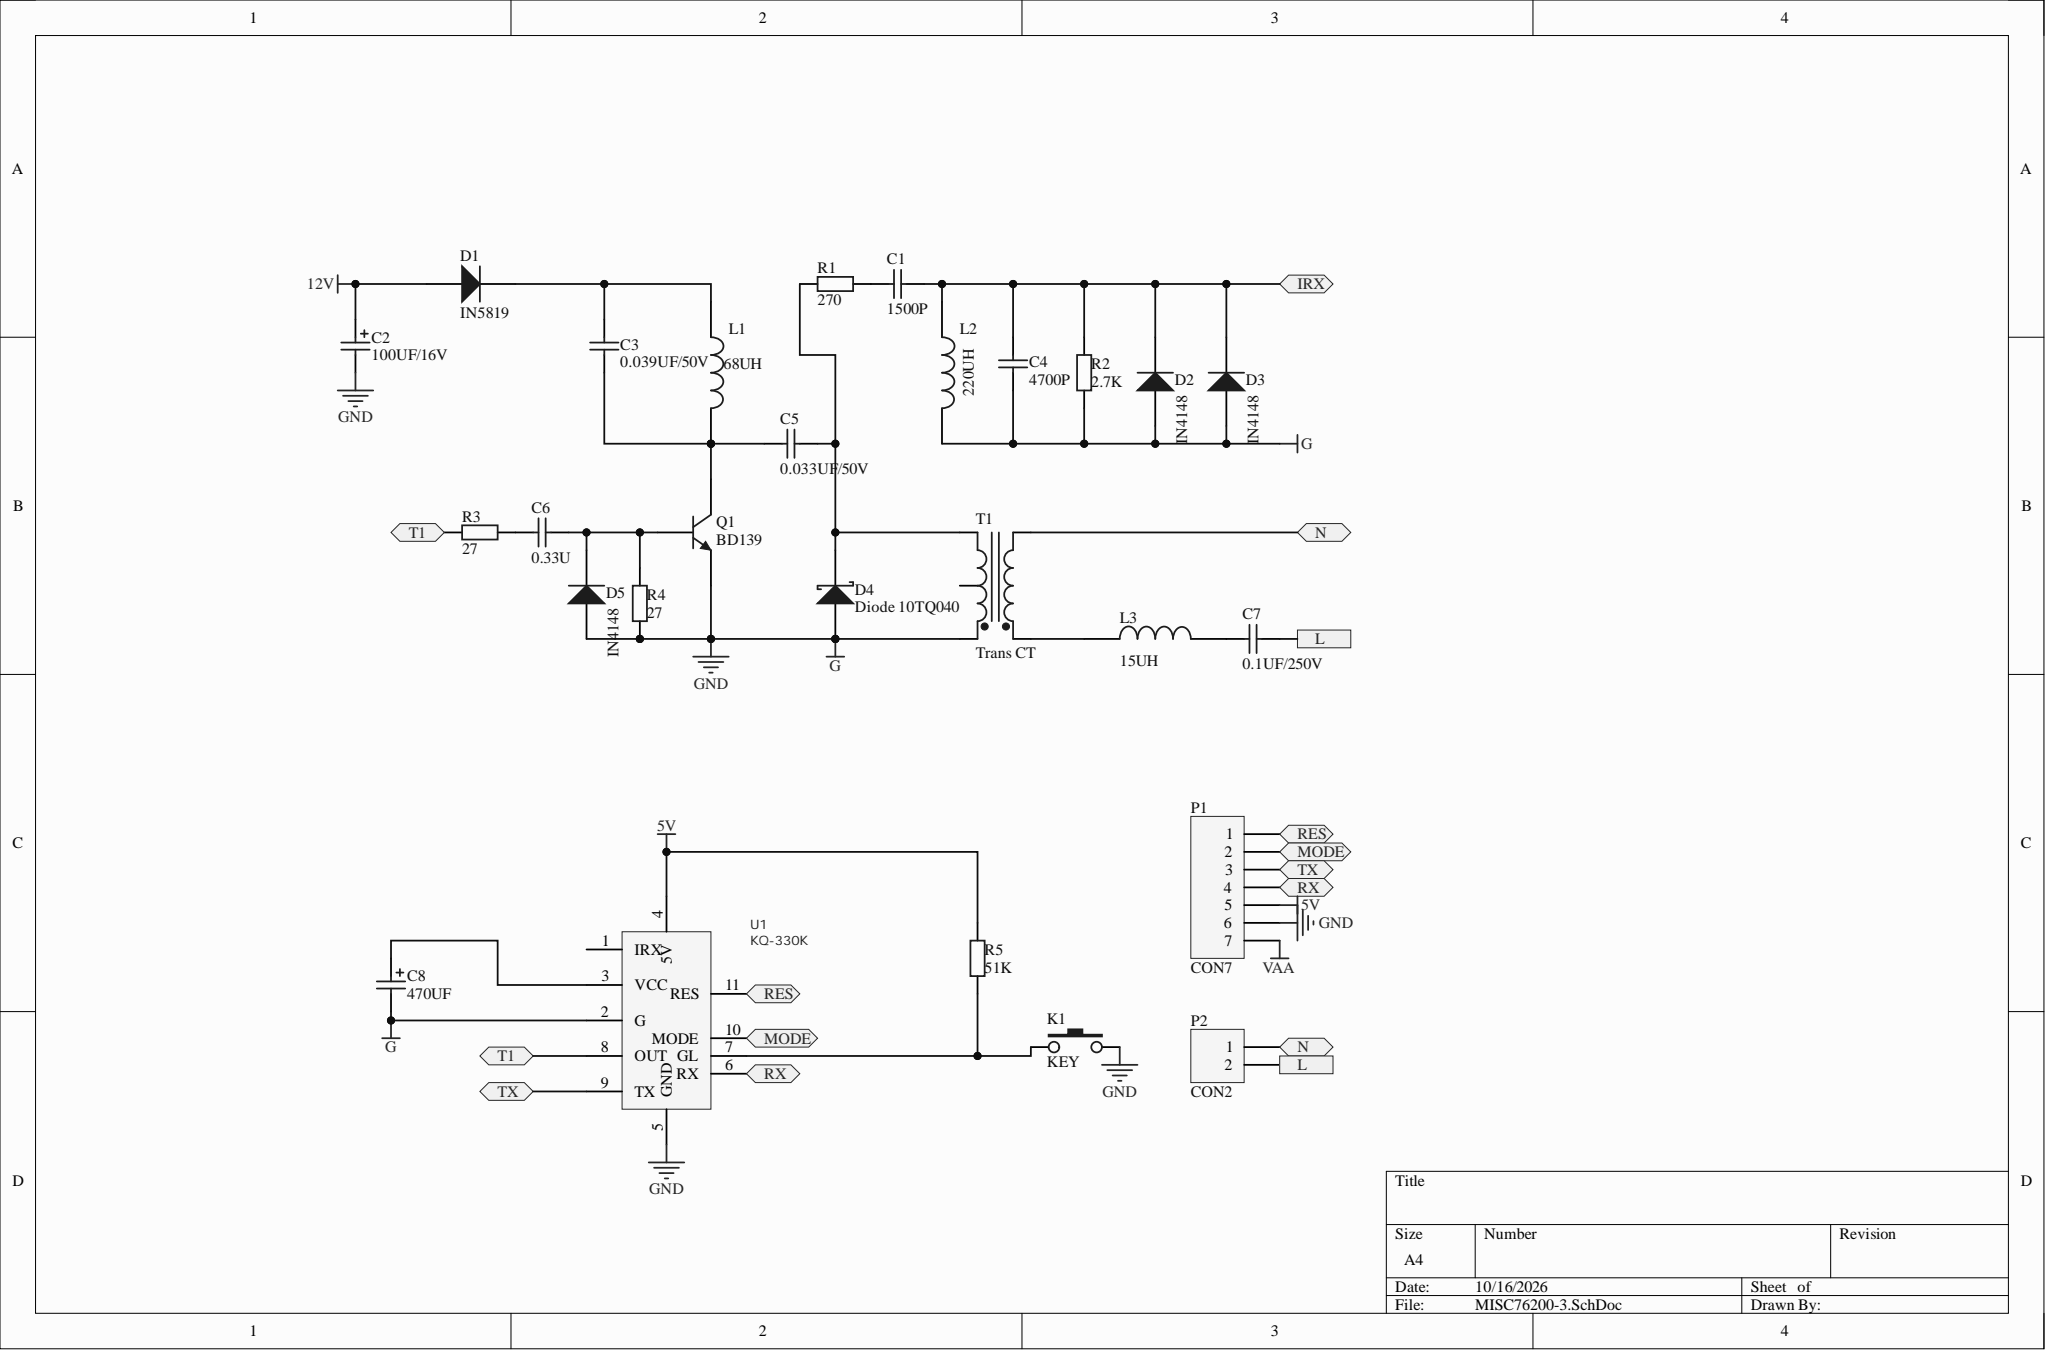Circuit board | Altium Designer | 27 parts | 21 nets
Bill of materials:
Comment,Description,Designator,Footprint,LibRef,Quantity
"1500P","Capacitor","C1","RAD-0.3","Cap","1"
"100UF/16V","Polarized Capacitor (Axial)","C2","POLAR0.8","Cap Pol2","1"
"0.039UF/50V","Capacitor","C3","RAD-0.3","Cap","1"
"4700P","Capacitor","C4","RAD-0.3","Cap","1"
"0.033UF/50V","Capacitor","C5","RAD-0.3","Cap","1"
"0.33U","Capacitor","C6","RAD-0.3","Cap","1"
"0.1UF/250V","Capacitor","C7","RAD-0.3","Cap","1"
"470UF","Polarized Capacitor (Axial)","C8","POLAR0.8","Cap Pol2","1"
"IN5819","Computer Diode","D1","DO-35A","Diode 1N4149","1"
"IN4148","Computer Diode","D2, D3, D5","DO-35A","Diode 1N4149","3"
"Diode 10TQ040","Schottky Rectifier","D4","TO-220AC","Diode 10TQ040","1"
"KEY","","K1","DIP-3X6X4.3","KEY","1"
"68UH","INDUCTOR","L1","AL0204","INDUCTOR","1"
"220UH","INDUCTOR","L2","AL0204","INDUCTOR","1"
"15UH","INDUCTOR","L3","AL0204","INDUCTOR","1"
"CON7","Header, 7-Pin","P1","HDR1X7","Header 7","1"
"CON2","Header, 2-Pin","P2","HDR1X2","Header 2","1"
"BD139","NPN Bipolar Transistor","Q1","TO-226-AA","NPN","1"
"270","Resistor","R1","AXIAL-0.4","Res2","1"
"2.7K","Resistor","R2","AXIAL-0.4","Res2","1"
"27","Resistor","R3, R4","AXIAL-0.4","Res2","2"
"51K","Resistor","R5","AXIAL-0.4","Res2","1"
"Trans CT","Center-Tapped Transformer (Coupled Inductor Model)","T1","TRF_5","Trans CT","1"
"KQ-330K","","U1","20130-10PIN","20130-10PIN","1"
Netlist (Protel format):
[
C1
RAD-0.3
1500P



]
[
C2
POLAR0.8
100UF/16V



]
[
C3
RAD-0.3
0.039UF/50V



]
[
C4
RAD-0.3
4700P



]
[
C5
RAD-0.3
0.033UF/50V



]
[
C6
RAD-0.3
0.33U



]
[
C7
RAD-0.3
0.1UF/250V



]
[
C8
POLAR0.8
470UF



]
[
D1
DO-35A
IN5819



]
[
D2
DO-35A
IN4148



]
[
D3
DO-35A
IN4148



]
[
D4
TO-220AC
Diode 10TQ040



]
[
D5
DO-35A
IN4148



]
[
K1
DIP-3X6X4.3
KEY



]
[
L1
AL0204
68UH



]
[
L2
AL0204
220UH



]
[
L3
AL0204
15UH



]
[
P1
HDR1X7
CON7



]
[
P2
HDR1X2
CON2



]
[
Q1
TO-226-AA
BD139



]
[
R1
AXIAL-0.4
270



]
[
R2
AXIAL-0.4
2.7K



]
[
R3
AXIAL-0.4
27



]
[
R4
AXIAL-0.4
27



]
[
R5
AXIAL-0.4
51K



]
[
T1
TRF_5
Trans CT



]
[
U1
20130-10PIN
KQ-330K



]
(
NetR3_1
R3-1
U1-8
)
(
NetP2_1
P2-1
T1-2
)
(
NetP1_4
P1-4
U1-6
)
(
NetP1_3
P1-3
U1-9
)
(
NetP1_2
P1-2
U1-10
)
(
NetP1_1
P1-1
U1-11
)
(
NetL3_1
L3-1
T1-1
)
(
NetK1_1
K1-1
R5-1
U1-7
)
(
NetC8_1
C8-1
U1-3
)
(
NetC7_2
C7-2
L3-2
)
(
NetC7_1
C7-1
P2-2
)
(
NetC6_2
C6-2
R3-2
)
(
NetC6_1
C6-1
D5-2
Q1-2
R4-2
)
(
NetC5_1
C5-1
D4-1
R1-1
T1-5
)
(
NetC3_2
C3-2
D1-2
L1-1
)
(
NetC3_1
C3-1
C5-2
L1-2
Q1-1
)
(
NetC1_2
C1-2
R1-2
)
(
NetC1_1
C1-1
C4-1
D2-2
D3-2
L2-1
R2-2
)
(
G
C2-2
C4-2
C8-2
D2-1
D3-1
D4-3
D5-1
K1-3
L2-2
P1-6
Q1-3
R2-1
R4-1
T1-3
U1-2
U1-5
)
(
12V
C2-1
D1-1
)
(
5V
P1-5
R5-2
U1-4
)